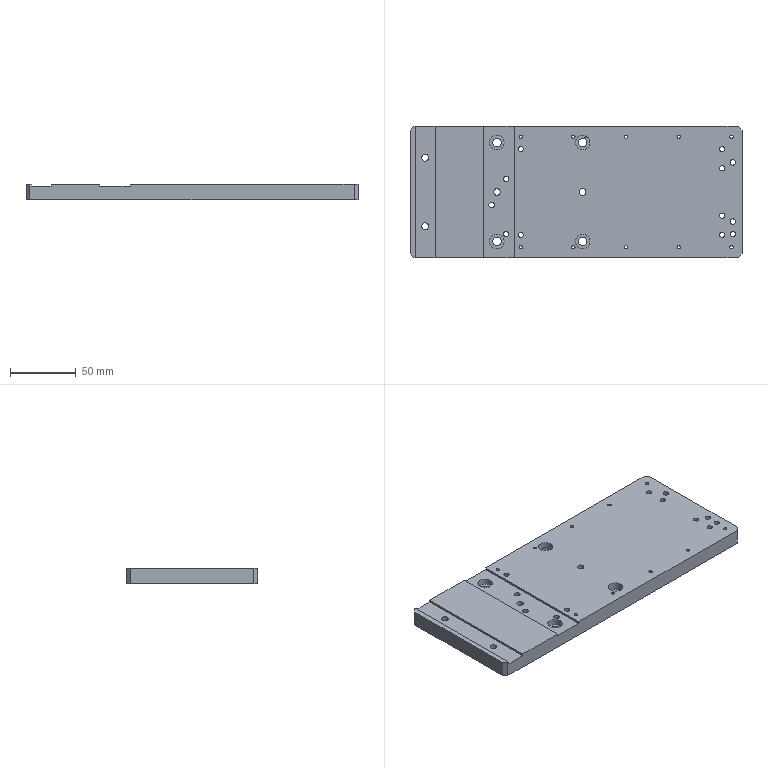CAM job | NX | 3-axis milling, drilling | part box 252 x 100 x 12 mm | stock box 257 x 100 x 15 mm
Tools:
number,name,description,diameter,corner_radius,flute_length,length,flutes
6,D6,平底铣刀-粗,6.0,0.0,25.0,75.0,2
9,D10,平底铣刀-粗,10.0,0.0,35.0,75.0,2
7,D6-J,平底铣刀-精,6.0,0.0,25.0,75.0,2
10,D10-J,平底铣刀-精,10.0,0.0,35.0,75.0,2
1,D80R0.8_FLYCUTTER,圆鼻刀-粗,80.0,0.8,50.0,75.0,2
1,D80R0.8_FLYCUTTER-J,圆鼻刀-精,80.0,0.8,50.0,75.0,2
2,D6_CHAMFERCUTTER,倒角刀,6.0,0.0,3.0,25.0,2
20,M3X0.5,丝锥,2.5,0.0,35.0,50.0,2
22,M5X0.8,丝锥,4.2,0.0,35.0,50.0,2
23,M6X1.0,丝锥,5.0,0.0,35.0,50.0,2
21,D4_REAMER,Drilling Tool,4.0,0.0,75.0,100.0,6
24,D5_REAMER,Drilling Tool,5.0,0.0,75.0,100.0,6
12,ZT2.6,钻头,2.6,0.0,35.0,50.0,2
15,ZT5.1,钻头,5.1,0.0,35.0,50.0,2
19,DRILL6.6,Drilling Tool,6.6,0.0,35.0,50.0,2
17,ZT3.9,Drilling Tool,3.9,0.0,35.0,50.0,2
18,ZT4.9,Drilling Tool,4.9,0.0,35.0,50.0,2
14,ZT4.3,Drilling Tool,4.3,0.0,50.0,75.0,4
Operations:
program,operation,operation_type,tool,method,geometry_group,spindle_rpm,surface_speed,feed_per_tooth,feed_cut,feed_plunge,cut_length_mm,path_length_mm,cut_time_min,machine_time_min
B,BOTTOMWALL_FACEROUGH_COPY,VolumeBased25DMillingOperation,D80R0.8_FLYCUTTER,ZLEVELROUGH-DEPTHK-STEPG,W-B,2800.0,703.696,0.5357,3000.0,100.0,3653.487,3926.711,1.218,1.245
B,BOTTOMWALL_FACEFINISH_COPY,VolumeBased25DMillingOperation,D80R0.8_FLYCUTTER-J,SIDEFINISH-DEPTHK-STEPG,W-B,4000.0,1005.28,0.125,1000.0,100.0,730.11,826.11,0.7301,0.7397
B,NG_DRILLCHAMFER_3,Operation,D6_CHAMFERCUTTER,METHOD,W-B,8000.0,150.796,0.0625,1000.0,0.0,47.5,626.952,0.0475,0.1054
B,NG_DRILLCHAMFER_7,Operation,D6_CHAMFERCUTTER,METHOD,W-B,8000.0,150.796,0.0625,1000.0,0.0,42.4,509.609,0.0424,0.0891
B,NG_DRILLCHAMFER_8,Operation,D6_CHAMFERCUTTER,METHOD,W-B,8000.0,150.796,0.0625,1000.0,0.0,11.6,191.269,0.0116,0.0296
B,NG_DRILLCHAMFER_9,Operation,D6_CHAMFERCUTTER,METHOD,W-B,8000.0,150.796,0.0625,1000.0,0.0,22.8,395.201,0.0228,0.06
B,PLANARMILL_CHAMFER_4,PlanarMilling,D6_CHAMFERCUTTER,METHOD,W-B,8000.0,150.796,0.0375,600.0,100.0,38.393,295.813,0.064,0.0897
B,PLANARMILL_CHAMFER_5,PlanarMilling,D6_CHAMFERCUTTER,METHOD,W-B,8000.0,150.796,0.075,1200.0,100.0,81.784,696.231,0.0682,0.1296
B,C0.3_CLOSEDCONTOURCHAMFER6X45L_COPY,PlanarMilling,D6_CHAMFERCUTTER,CLIMBSURF_CHAMFER-DEPTH0-STEPG,W-B,7000.0,131.0,0.1071,1500.0,100.0,714.499,810.499,0.4763,0.4859
A,TOPFACE,FaceMilling,D80R0.8_FLYCUTTER,SIDEFINISH-DEPTHK-STEPG,W-A,4500.0,1385.0,0.1667,1500.0,100.0,1100.0,1196.0,0.7333,0.7429
A,PROFILEROUGH_2,VolumeBased25DMillingOperation,D10,METHOD,W-A,8000.0,251.327,0.375,6000.0,80.0,12394.758,12505.258,2.066,2.077
A,BOTTOMWALLROUGH_1,VolumeBased25DMillingOperation,D10,METHOD,W-A,9000.0,282.743,0.3333,6000.0,100.0,1322.1,1439.802,0.2204,0.2321
A,BOTTOMWALLROUGH_2,VolumeBased25DMillingOperation,D10,METHOD,W-A,9000.0,282.743,0.3333,6000.0,100.0,666.6,784.502,0.1111,0.1229
A,SPOTDRILL-DEPTH0.8,Operation,D6_CHAMFERCUTTER,NONE,W-A,8000.0,150.796,0.0312,500.0,90.0,54.0,910.969,0.108,0.1937
A,THRUHOLE-M3TAPDRILL,Operation,ZT2.6,NONE,W-A,3000.0,23.562,0.05,300.0,90.0,190.0,893.106,0.6333,0.7036
A,THRUHOLE-PRECISION4.0_PREDRILL,Operation,ZT3.9,NONE,W-A,3000.0,36.757,0.0417,250.0,90.0,135.507,681.976,0.542,0.5967
A,THRUHOLE-M5TAPDRILL,Operation,ZT4.3,NONE,W-A,3000.0,39.584,0.0583,350.0,90.0,84.0,512.83,0.24,0.2829
A,THRUHOLE-PRECISION6.0_PREDRILL,Operation,ZT4.9,NONE,W-A,2500.0,38.484,0.05,250.0,90.0,33.329,234.206,0.1333,0.1534
A,THRUHOLE-M6TAPDRILL,Operation,ZT5.1,NONE,W-A,2800.0,44.862,0.0625,350.0,90.0,38.064,232.138,0.1088,0.1282
A,COUNTERBORE-DRILL_SEG0,Operation,DRILL6.6,NONE,W-A,1200.0,24.881,0.0625,150.0,90.0,64.621,437.299,0.4308,0.4681
A,HOLEMILL_ROUGH_D6_1,CylinderMilling,D6,NONE,W-A,8000.0,150.796,0.075,1200.0,100.0,461.666,748.466,0.3847,0.4134
A,HOLEMILL_ROUGH_D6_2,CylinderMilling,D6,NONE,W-A,8000.0,150.796,0.075,1200.0,100.0,371.138,660.938,0.3093,0.3383
A,HOLEMILL_FINISH_D6_1,CylinderMilling,D6-J,FINISH-STEPDEPTH-OFF,W-A,8000.0,150.796,0.0312,500.0,100.0,89.231,377.031,0.1785,0.2072
A,HOLEMILL_FINISH_D6_2,CylinderMilling,D6-J,FINISH-STEPDEPTH-OFF,W-A,8000.0,150.796,0.0312,500.0,100.0,79.34,370.14,0.1587,0.1878
A,BOTTOMFINISH_1,VolumeBased25DMillingOperation,D10-J,METHOD,W-A,9000.0,169.646,0.0833,1500.0,100.0,446.1,548.1,0.2974,0.3076
A,BOTTOMFINISH_2,VolumeBased25DMillingOperation,D10-J,METHOD,W-A,9000.0,169.646,0.0833,1500.0,100.0,228.9,330.9,0.1526,0.1628
A,NG_DRILLCHAMFER_1,Operation,D6_CHAMFERCUTTER,METHOD,W-A,8000.0,150.796,0.0312,500.0,0.0,47.5,626.952,0.095,0.1529
A,NG_DRILLCHAMFER_2,Operation,D6_CHAMFERCUTTER,METHOD,W-A,8000.0,150.796,0.0312,500.0,0.0,42.4,511.592,0.0848,0.1317
A,PLANARMILL_CHAMFER_1,PlanarMilling,D6_CHAMFERCUTTER,METHOD,W-A,8000.0,150.796,0.0312,500.0,100.0,36.041,284.428,0.0721,0.0969
A,PLANARMILL_CHAMFER_2,PlanarMilling,D6_CHAMFERCUTTER,METHOD,W-A,8000.0,150.796,0.0312,500.0,100.0,18.482,119.481,0.037,0.0471
A,PLANARMILL_CHAMFER_3,PlanarMilling,D6_CHAMFERCUTTER,METHOD,W-A,8000.0,150.796,0.0312,500.0,100.0,40.382,302.892,0.0808,0.107
A,NG_DRILLCHAMFER_4,Operation,D6_CHAMFERCUTTER,METHOD,W-A,8000.0,150.796,0.0625,1000.0,0.0,42.4,511.592,0.0424,0.0893
A,NG_DRILLCHAMFER_5,Operation,D6_CHAMFERCUTTER,METHOD,W-A,8000.0,150.796,0.0625,1000.0,0.0,11.6,192.856,0.0116,0.0297
A,NG_DRILLCHAMFER_6,Operation,D6_CHAMFERCUTTER,METHOD,W-A,8000.0,150.796,0.0625,1000.0,0.0,22.8,396.734,0.0228,0.0602
A,PLANARDEBURR6X45L_COPY,SurfaceContour,D6_CHAMFERCUTTER,CLIMBSURF_CHAMFER-DEPTH0-STEPG,W-A,6500.0,122.519,0.1154,1500.0,100.0,1446.125,3223.1,0.9641,1.142
A,REAM,Operation,D4_REAMER,METHOD,W-A,500.0,6.283,0.0167,50.0,0.0,112.0,633.228,2.24,2.292
A,REAM_2,Operation,D5_REAMER,METHOD,W-A,500.0,7.854,0.0167,50.0,0.0,28.0,222.008,0.56,0.5794
A,THRUHOLE-TAPM3,Operation,M3X0.5,METHOD,W-A,800.0,6.283,0.0003,0.5,90.0,160.0,833.106,320.0,320.067
A,THRUHOLE-TAPM5,Operation,M5X0.8,METHOD,W-A,500.0,6.597,0.0008,0.8,90.0,66.0,475.315,82.5,82.541
A,THRUHOLE-TAPM6,Operation,M6X1.0,METHOD,W-A,500.0,7.854,0.001,1.0,90.0,30.0,216.01,30.0,30.019
A,BOTTOMSIDEFINISH_3,VolumeBased25DMillingOperation,D10-J,METHOD,W-A,9000.0,282.743,0.0556,1000.0,100.0,236.533,338.523,0.2365,0.2467
A,BOTTOMSIDEFINISH_4,VolumeBased25DMillingOperation,D10-J,METHOD,W-A,9000.0,282.743,0.0556,1000.0,100.0,228.533,330.523,0.2285,0.2387
A,PROFILESEMIFINISH_2,VolumeBased25DMillingOperation,D6-J,METHOD,W-A,9000.0,169.646,0.0667,1200.0,100.0,720.736,843.736,0.6006,0.6129
A,BOTTOMWALL_SIDEFINISH-MID_COPY,VolumeBased25DMillingOperation,D6-J,SIDEFINISH-DEPTHK-STEPG,W-A,8000.0,150.792,0.0625,1000.0,100.0,516.455,708.605,0.5165,0.5357